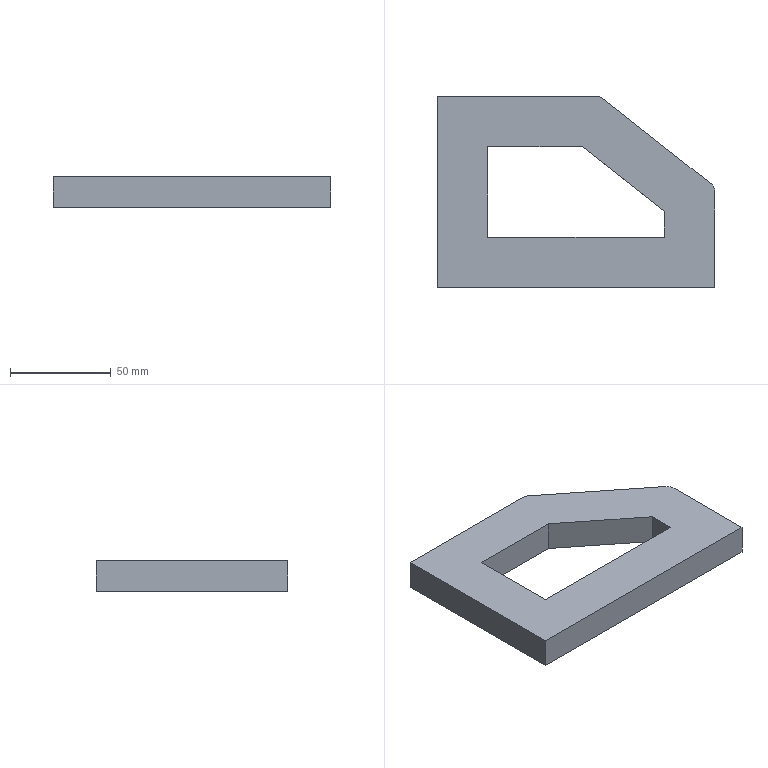Part | STEP file | ASND-0110-Part 14989898 | 1 solid | 16 faces | box 137.7 x 95 x 15 mm | volume 127568 mm3 | plane 12 | cylinder 4 | commonest cylinder face diameters 10 x4
STEP:
#1=CARTESIAN_POINT('',(0.,0.,0.));
#2=DIRECTION('',(0.,0.,1.));
#3=DIRECTION('',(1.,0.,0.));
#4=AXIS2_PLACEMENT_3D('',#1,#2,#3);
#5=CARTESIAN_POINT('',(78.964,95.,15.));
#6=VERTEX_POINT('',#5);
#7=CARTESIAN_POINT('',(80.604,94.723,15.));
#8=VERTEX_POINT('',#7);
#9=CARTESIAN_POINT('',(78.964,90.,15.));
#10=DIRECTION('',(0.,0.,-1.));
#11=DIRECTION('',(0.328,0.9447,0.));
#12=AXIS2_PLACEMENT_3D('',#9,#10,#11);
#13=CIRCLE('',#12,5.);
#14=CARTESIAN_POINT('',(78.964,90.,20.));
#15=DIRECTION('',(0.,0.,-1.));
#16=DIRECTION('',(0.328,0.9447,0.));
#17=AXIS2_PLACEMENT_3D('',#14,#15,#16);
#18=CYLINDRICAL_SURFACE('',#17,5.);
#19=CARTESIAN_POINT('',(0.,5.));
#20=DIRECTION('',(1.,0.));
#21=VECTOR('',#20,1.);
#22=LINE('',#19,#21);
#23=(GEOMETRIC_REPRESENTATION_CONTEXT(2)PARAMETRIC_REPRESENTATION_CONTEXT()REPRESENTATION_CONTEXT('',''));
#24=DEFINITIONAL_REPRESENTATION('',(#22),#23);
#25=PCURVE('',#18,#24);
#26=CARTESIAN_POINT('',(0.,0.,15.));
#27=DIRECTION('',(0.,0.,-1.));
#28=DIRECTION('',(0.7071,0.7071,0.));
#29=AXIS2_PLACEMENT_3D('',#26,#27,#28);
#30=PLANE('',#29);
#31=CARTESIAN_POINT('',(119.476,-7.803));
#32=DIRECTION('',(0.8999,-0.4361));
#33=AXIS2_PLACEMENT_2D('',#31,#32);
#34=CIRCLE('',#33,5.);
#35=(GEOMETRIC_REPRESENTATION_CONTEXT(2)PARAMETRIC_REPRESENTATION_CONTEXT()REPRESENTATION_CONTEXT('',''));
#36=DEFINITIONAL_REPRESENTATION('',(#34),#35);
#37=PCURVE('',#30,#36);
#38=SURFACE_CURVE('',#13,(#25,#37),.PCURVE_S1.);
#39=EDGE_CURVE('',#6,#8,#38,.T.);
#40=ORIENTED_EDGE('',*,*,#39,.T.);
#41=CARTESIAN_POINT('',(80.604,94.723,0.));
#42=VERTEX_POINT('',#41);
#43=CARTESIAN_POINT('',(80.604,94.723,20.));
#44=DIRECTION('',(0.,0.,-1.));
#45=VECTOR('',#44,1.);
#46=LINE('',#43,#45);
#47=CARTESIAN_POINT('',(6.283,0.));
#48=DIRECTION('',(0.,1.));
#49=VECTOR('',#48,1.);
#50=LINE('',#47,#49);
#51=(GEOMETRIC_REPRESENTATION_CONTEXT(2)PARAMETRIC_REPRESENTATION_CONTEXT()REPRESENTATION_CONTEXT('',''));
#52=DEFINITIONAL_REPRESENTATION('',(#50),#51);
#53=PCURVE('',#18,#52);
#54=CARTESIAN_POINT('',(78.964,90.,20.));
#55=DIRECTION('',(0.,0.,-1.));
#56=DIRECTION('',(0.328,0.9447,0.));
#57=AXIS2_PLACEMENT_3D('',#54,#55,#56);
#58=CYLINDRICAL_SURFACE('',#57,5.);
#59=CARTESIAN_POINT('',(0.,0.));
#60=DIRECTION('',(0.,1.));
#61=VECTOR('',#60,1.);
#62=LINE('',#59,#61);
#63=(GEOMETRIC_REPRESENTATION_CONTEXT(2)PARAMETRIC_REPRESENTATION_CONTEXT()REPRESENTATION_CONTEXT('',''));
#64=DEFINITIONAL_REPRESENTATION('',(#62),#63);
#65=PCURVE('',#58,#64);
#66=SURFACE_CURVE('',#46,(#53,#65),.PCURVE_S1.);
#67=EDGE_CURVE('',#8,#42,#66,.T.);
#68=ORIENTED_EDGE('',*,*,#67,.T.);
#69=CARTESIAN_POINT('',(78.964,95.,0.));
#70=VERTEX_POINT('',#69);
#71=CARTESIAN_POINT('',(78.964,90.,0.));
#72=DIRECTION('',(0.,0.,1.));
#73=DIRECTION('',(0.328,0.9447,0.));
#74=AXIS2_PLACEMENT_3D('',#71,#72,#73);
#75=CIRCLE('',#74,5.);
#76=CARTESIAN_POINT('',(6.283,20.));
#77=DIRECTION('',(-1.,0.));
#78=VECTOR('',#77,1.);
#79=LINE('',#76,#78);
#80=(GEOMETRIC_REPRESENTATION_CONTEXT(2)PARAMETRIC_REPRESENTATION_CONTEXT()REPRESENTATION_CONTEXT('',''));
#81=DEFINITIONAL_REPRESENTATION('',(#79),#80);
#82=PCURVE('',#18,#81);
#83=CARTESIAN_POINT('',(0.,0.,0.));
#84=DIRECTION('',(0.,0.,-1.));
#85=DIRECTION('',(0.7071,0.7071,0.));
#86=AXIS2_PLACEMENT_3D('',#83,#84,#85);
#87=PLANE('',#86);
#88=CARTESIAN_POINT('',(123.975,-9.984));
#89=CARTESIAN_POINT('',(120.199,-17.777));
#90=CARTESIAN_POINT('',(115.338,-10.61));
#91=CARTESIAN_POINT('',(110.477,-3.443));
#92=CARTESIAN_POINT('',(119.114,-2.817));
#93=CARTESIAN_POINT('',(127.752,-2.191));
#94=CARTESIAN_POINT('',(123.975,-9.984));
#95=(BOUNDED_CURVE()B_SPLINE_CURVE(2,(#88,#89,#90,#91,#92,#93,#94),.UNSPECIFIED.,.T.,.F.)B_SPLINE_CURVE_WITH_KNOTS((1,2,2,2,2,1),(-2.094,0.,2.094,4.189,6.283,8.378),.UNSPECIFIED.)CURVE()GEOMETRIC_REPRESENTATION_ITEM()RATIONAL_B_SPLINE_CURVE((1.,0.5,1.,0.5,1.,0.5,1.))REPRESENTATION_ITEM(''));
#96=(GEOMETRIC_REPRESENTATION_CONTEXT(2)PARAMETRIC_REPRESENTATION_CONTEXT()REPRESENTATION_CONTEXT('',''));
#97=DEFINITIONAL_REPRESENTATION('',(#95),#96);
#98=PCURVE('',#87,#97);
#99=SURFACE_CURVE('',#75,(#82,#98),.PCURVE_S1.);
#100=EDGE_CURVE('',#42,#70,#99,.T.);
#101=ORIENTED_EDGE('',*,*,#100,.T.);
#102=CARTESIAN_POINT('',(78.964,95.,20.));
#103=DIRECTION('',(0.,0.,1.));
#104=VECTOR('',#103,1.);
#105=LINE('',#102,#104);
#106=CARTESIAN_POINT('',(5.949,0.));
#107=DIRECTION('',(0.,-1.));
#108=VECTOR('',#107,1.);
#109=LINE('',#106,#108);
#110=(GEOMETRIC_REPRESENTATION_CONTEXT(2)PARAMETRIC_REPRESENTATION_CONTEXT()REPRESENTATION_CONTEXT('',''));
#111=DEFINITIONAL_REPRESENTATION('',(#109),#110);
#112=PCURVE('',#18,#111);
#113=CARTESIAN_POINT('',(0.,95.,20.));
#114=DIRECTION('',(0.,-1.,0.));
#115=DIRECTION('',(0.7071,0.,0.7071));
#116=AXIS2_PLACEMENT_3D('',#113,#114,#115);
#117=PLANE('',#116);
#118=CARTESIAN_POINT('',(55.836,-55.836));
#119=DIRECTION('',(0.7071,0.7071));
#120=VECTOR('',#119,1.);
#121=LINE('',#118,#120);
#122=(GEOMETRIC_REPRESENTATION_CONTEXT(2)PARAMETRIC_REPRESENTATION_CONTEXT()REPRESENTATION_CONTEXT('',''));
#123=DEFINITIONAL_REPRESENTATION('',(#121),#122);
#124=PCURVE('',#117,#123);
#125=SURFACE_CURVE('',#105,(#112,#124),.PCURVE_S1.);
#126=EDGE_CURVE('',#70,#6,#125,.T.);
#127=ORIENTED_EDGE('',*,*,#126,.T.);
#128=EDGE_LOOP('',(#40,#68,#101,#127));
#129=FACE_BOUND('',#128,.T.);
#130=ADVANCED_FACE('',(#129),#18,.T.);
#131=CARTESIAN_POINT('',(135.798,51.501,15.));
#132=VERTEX_POINT('',#131);
#133=CARTESIAN_POINT('',(137.2,49.757,15.));
#134=VERTEX_POINT('',#133);
#135=CARTESIAN_POINT('',(132.7,47.577,15.));
#136=DIRECTION('',(0.,0.,-1.));
#137=DIRECTION('',(0.8999,0.4361,0.));
#138=AXIS2_PLACEMENT_3D('',#135,#136,#137);
#139=CIRCLE('',#138,5.);
#140=CARTESIAN_POINT('',(132.7,47.577,20.));
#141=DIRECTION('',(0.,0.,-1.));
#142=DIRECTION('',(0.8999,0.4361,0.));
#143=AXIS2_PLACEMENT_3D('',#140,#141,#142);
#144=CYLINDRICAL_SURFACE('',#143,5.);
#145=CARTESIAN_POINT('',(0.,5.));
#146=DIRECTION('',(1.,0.));
#147=VECTOR('',#146,1.);
#148=LINE('',#145,#147);
#149=(GEOMETRIC_REPRESENTATION_CONTEXT(2)PARAMETRIC_REPRESENTATION_CONTEXT()REPRESENTATION_CONTEXT('',''));
#150=DEFINITIONAL_REPRESENTATION('',(#148),#149);
#151=PCURVE('',#144,#150);
#152=CARTESIAN_POINT('',(127.475,60.191));
#153=DIRECTION('',(0.9447,0.328));
#154=AXIS2_PLACEMENT_2D('',#152,#153);
#155=CIRCLE('',#154,5.);
#156=(GEOMETRIC_REPRESENTATION_CONTEXT(2)PARAMETRIC_REPRESENTATION_CONTEXT()REPRESENTATION_CONTEXT('',''));
#157=DEFINITIONAL_REPRESENTATION('',(#155),#156);
#158=PCURVE('',#30,#157);
#159=SURFACE_CURVE('',#139,(#151,#158),.PCURVE_S1.);
#160=EDGE_CURVE('',#132,#134,#159,.T.);
#161=ORIENTED_EDGE('',*,*,#160,.T.);
#162=CARTESIAN_POINT('',(137.2,49.757,0.));
#163=VERTEX_POINT('',#162);
#164=CARTESIAN_POINT('',(137.2,49.757,20.));
#165=DIRECTION('',(0.,0.,-1.));
#166=VECTOR('',#165,1.);
#167=LINE('',#164,#166);
#168=CARTESIAN_POINT('',(6.283,0.));
#169=DIRECTION('',(0.,1.));
#170=VECTOR('',#169,1.);
#171=LINE('',#168,#170);
#172=(GEOMETRIC_REPRESENTATION_CONTEXT(2)PARAMETRIC_REPRESENTATION_CONTEXT()REPRESENTATION_CONTEXT('',''));
#173=DEFINITIONAL_REPRESENTATION('',(#171),#172);
#174=PCURVE('',#144,#173);
#175=CARTESIAN_POINT('',(132.7,47.577,20.));
#176=DIRECTION('',(0.,0.,-1.));
#177=DIRECTION('',(0.8999,0.4361,0.));
#178=AXIS2_PLACEMENT_3D('',#175,#176,#177);
#179=CYLINDRICAL_SURFACE('',#178,5.);
#180=CARTESIAN_POINT('',(0.,0.));
#181=DIRECTION('',(0.,1.));
#182=VECTOR('',#181,1.);
#183=LINE('',#180,#182);
#184=(GEOMETRIC_REPRESENTATION_CONTEXT(2)PARAMETRIC_REPRESENTATION_CONTEXT()REPRESENTATION_CONTEXT('',''));
#185=DEFINITIONAL_REPRESENTATION('',(#183),#184);
#186=PCURVE('',#179,#185);
#187=SURFACE_CURVE('',#167,(#174,#186),.PCURVE_S1.);
#188=EDGE_CURVE('',#134,#163,#187,.T.);
#189=ORIENTED_EDGE('',*,*,#188,.T.);
#190=CARTESIAN_POINT('',(135.798,51.501,0.));
#191=VERTEX_POINT('',#190);
#192=CARTESIAN_POINT('',(132.7,47.577,0.));
#193=DIRECTION('',(0.,0.,1.));
#194=DIRECTION('',(0.8999,0.4361,0.));
#195=AXIS2_PLACEMENT_3D('',#192,#193,#194);
#196=CIRCLE('',#195,5.);
#197=CARTESIAN_POINT('',(6.283,20.));
#198=DIRECTION('',(-1.,0.));
#199=VECTOR('',#198,1.);
#200=LINE('',#197,#199);
#201=(GEOMETRIC_REPRESENTATION_CONTEXT(2)PARAMETRIC_REPRESENTATION_CONTEXT()REPRESENTATION_CONTEXT('',''));
#202=DEFINITIONAL_REPRESENTATION('',(#200),#201);
#203=PCURVE('',#144,#202);
#204=CARTESIAN_POINT('',(132.199,61.831));
#205=CARTESIAN_POINT('',(135.039,53.65));
#206=CARTESIAN_POINT('',(126.533,55.281));
#207=CARTESIAN_POINT('',(118.028,56.911));
#208=CARTESIAN_POINT('',(123.693,63.462));
#209=CARTESIAN_POINT('',(129.358,70.012));
#210=CARTESIAN_POINT('',(132.199,61.831));
#211=(BOUNDED_CURVE()B_SPLINE_CURVE(2,(#204,#205,#206,#207,#208,#209,#210),.UNSPECIFIED.,.T.,.F.)B_SPLINE_CURVE_WITH_KNOTS((1,2,2,2,2,1),(-2.094,0.,2.094,4.189,6.283,8.378),.UNSPECIFIED.)CURVE()GEOMETRIC_REPRESENTATION_ITEM()RATIONAL_B_SPLINE_CURVE((1.,0.5,1.,0.5,1.,0.5,1.))REPRESENTATION_ITEM(''));
#212=(GEOMETRIC_REPRESENTATION_CONTEXT(2)PARAMETRIC_REPRESENTATION_CONTEXT()REPRESENTATION_CONTEXT('',''));
#213=DEFINITIONAL_REPRESENTATION('',(#211),#212);
#214=PCURVE('',#87,#213);
#215=SURFACE_CURVE('',#196,(#203,#214),.PCURVE_S1.);
#216=EDGE_CURVE('',#163,#191,#215,.T.);
#217=ORIENTED_EDGE('',*,*,#216,.T.);
#218=CARTESIAN_POINT('',(135.798,51.501,20.));
#219=DIRECTION('',(0.,0.,1.));
#220=VECTOR('',#219,1.);
#221=LINE('',#218,#220);
#222=CARTESIAN_POINT('',(5.832,0.));
#223=DIRECTION('',(0.,-1.));
#224=VECTOR('',#223,1.);
#225=LINE('',#222,#224);
#226=(GEOMETRIC_REPRESENTATION_CONTEXT(2)PARAMETRIC_REPRESENTATION_CONTEXT()REPRESENTATION_CONTEXT('',''));
#227=DEFINITIONAL_REPRESENTATION('',(#225),#226);
#228=PCURVE('',#144,#227);
#229=CARTESIAN_POINT('',(-52.3,200.,20.));
#230=DIRECTION('',(-0.6196,-0.7849,0.));
#231=DIRECTION('',(-0.6672,0.5267,0.5267));
#232=AXIS2_PLACEMENT_3D('',#229,#230,#231);
#233=PLANE('',#232);
#234=CARTESIAN_POINT('',(-203.713,-126.229));
#235=DIRECTION('',(0.5267,-0.85));
#236=VECTOR('',#235,1.);
#237=LINE('',#234,#236);
#238=(GEOMETRIC_REPRESENTATION_CONTEXT(2)PARAMETRIC_REPRESENTATION_CONTEXT()REPRESENTATION_CONTEXT('',''));
#239=DEFINITIONAL_REPRESENTATION('',(#237),#238);
#240=PCURVE('',#233,#239);
#241=SURFACE_CURVE('',#221,(#228,#240),.PCURVE_S1.);
#242=EDGE_CURVE('',#191,#132,#241,.T.);
#243=ORIENTED_EDGE('',*,*,#242,.T.);
#244=EDGE_LOOP('',(#161,#189,#217,#243));
#245=FACE_BOUND('',#244,.T.);
#246=ADVANCED_FACE('',(#245),#144,.T.);
#247=ORIENTED_EDGE('',*,*,#188,.F.);
#248=CARTESIAN_POINT('',(137.7,47.577,15.));
#249=VERTEX_POINT('',#248);
#250=CARTESIAN_POINT('',(132.7,47.577,15.));
#251=DIRECTION('',(0.,0.,-1.));
#252=DIRECTION('',(0.8999,0.4361,0.));
#253=AXIS2_PLACEMENT_3D('',#250,#251,#252);
#254=CIRCLE('',#253,5.);
#255=CARTESIAN_POINT('',(0.,5.));
#256=DIRECTION('',(1.,0.));
#257=VECTOR('',#256,1.);
#258=LINE('',#255,#257);
#259=(GEOMETRIC_REPRESENTATION_CONTEXT(2)PARAMETRIC_REPRESENTATION_CONTEXT()REPRESENTATION_CONTEXT('',''));
#260=DEFINITIONAL_REPRESENTATION('',(#258),#259);
#261=PCURVE('',#179,#260);
#262=CARTESIAN_POINT('',(127.475,60.191));
#263=DIRECTION('',(0.9447,0.328));
#264=AXIS2_PLACEMENT_2D('',#262,#263);
#265=CIRCLE('',#264,5.);
#266=(GEOMETRIC_REPRESENTATION_CONTEXT(2)PARAMETRIC_REPRESENTATION_CONTEXT()REPRESENTATION_CONTEXT('',''));
#267=DEFINITIONAL_REPRESENTATION('',(#265),#266);
#268=PCURVE('',#30,#267);
#269=SURFACE_CURVE('',#254,(#261,#268),.PCURVE_S1.);
#270=EDGE_CURVE('',#134,#249,#269,.T.);
#271=ORIENTED_EDGE('',*,*,#270,.T.);
#272=CARTESIAN_POINT('',(137.7,47.577,0.));
#273=VERTEX_POINT('',#272);
#274=CARTESIAN_POINT('',(137.7,47.577,20.));
#275=DIRECTION('',(0.,0.,-1.));
#276=VECTOR('',#275,1.);
#277=LINE('',#274,#276);
#278=CARTESIAN_POINT('',(0.4513,0.));
#279=DIRECTION('',(0.,1.));
#280=VECTOR('',#279,1.);
#281=LINE('',#278,#280);
#282=(GEOMETRIC_REPRESENTATION_CONTEXT(2)PARAMETRIC_REPRESENTATION_CONTEXT()REPRESENTATION_CONTEXT('',''));
#283=DEFINITIONAL_REPRESENTATION('',(#281),#282);
#284=PCURVE('',#179,#283);
#285=CARTESIAN_POINT('',(137.7,50.,20.));
#286=DIRECTION('',(-1.,0.,0.));
#287=DIRECTION('',(0.,0.7071,0.7071));
#288=AXIS2_PLACEMENT_3D('',#285,#286,#287);
#289=PLANE('',#288);
#290=CARTESIAN_POINT('',(-1.713,-1.713));
#291=DIRECTION('',(-0.7071,0.7071));
#292=VECTOR('',#291,1.);
#293=LINE('',#290,#292);
#294=(GEOMETRIC_REPRESENTATION_CONTEXT(2)PARAMETRIC_REPRESENTATION_CONTEXT()REPRESENTATION_CONTEXT('',''));
#295=DEFINITIONAL_REPRESENTATION('',(#293),#294);
#296=PCURVE('',#289,#295);
#297=SURFACE_CURVE('',#277,(#284,#296),.PCURVE_S1.);
#298=EDGE_CURVE('',#249,#273,#297,.T.);
#299=ORIENTED_EDGE('',*,*,#298,.T.);
#300=CARTESIAN_POINT('',(132.7,47.577,0.));
#301=DIRECTION('',(0.,0.,1.));
#302=DIRECTION('',(0.8999,0.4361,0.));
#303=AXIS2_PLACEMENT_3D('',#300,#301,#302);
#304=CIRCLE('',#303,5.);
#305=CARTESIAN_POINT('',(6.283,20.));
#306=DIRECTION('',(-1.,0.));
#307=VECTOR('',#306,1.);
#308=LINE('',#305,#307);
#309=(GEOMETRIC_REPRESENTATION_CONTEXT(2)PARAMETRIC_REPRESENTATION_CONTEXT()REPRESENTATION_CONTEXT('',''));
#310=DEFINITIONAL_REPRESENTATION('',(#308),#309);
#311=PCURVE('',#179,#310);
#312=CARTESIAN_POINT('',(132.199,61.831));
#313=CARTESIAN_POINT('',(135.039,53.65));
#314=CARTESIAN_POINT('',(126.533,55.281));
#315=CARTESIAN_POINT('',(118.028,56.911));
#316=CARTESIAN_POINT('',(123.693,63.462));
#317=CARTESIAN_POINT('',(129.358,70.012));
#318=CARTESIAN_POINT('',(132.199,61.831));
#319=(BOUNDED_CURVE()B_SPLINE_CURVE(2,(#312,#313,#314,#315,#316,#317,#318),.UNSPECIFIED.,.T.,.F.)B_SPLINE_CURVE_WITH_KNOTS((1,2,2,2,2,1),(-2.094,0.,2.094,4.189,6.283,8.378),.UNSPECIFIED.)CURVE()GEOMETRIC_REPRESENTATION_ITEM()RATIONAL_B_SPLINE_CURVE((1.,0.5,1.,0.5,1.,0.5,1.))REPRESENTATION_ITEM(''));
#320=(GEOMETRIC_REPRESENTATION_CONTEXT(2)PARAMETRIC_REPRESENTATION_CONTEXT()REPRESENTATION_CONTEXT('',''));
#321=DEFINITIONAL_REPRESENTATION('',(#319),#320);
#322=PCURVE('',#87,#321);
#323=SURFACE_CURVE('',#304,(#311,#322),.PCURVE_S1.);
#324=EDGE_CURVE('',#273,#163,#323,.T.);
#325=ORIENTED_EDGE('',*,*,#324,.T.);
#326=EDGE_LOOP('',(#247,#271,#299,#325));
#327=FACE_BOUND('',#326,.T.);
#328=ADVANCED_FACE('',(#327),#179,.T.);
#329=ORIENTED_EDGE('',*,*,#298,.F.);
#330=CARTESIAN_POINT('',(137.7,0.,15.));
#331=VERTEX_POINT('',#330);
#332=CARTESIAN_POINT('',(137.7,0.,15.));
#333=DIRECTION('',(0.,1.,0.));
#334=VECTOR('',#333,1.);
#335=LINE('',#332,#334);
#336=CARTESIAN_POINT('',(-38.891,-31.82));
#337=DIRECTION('',(0.7071,0.7071));
#338=VECTOR('',#337,1.);
#339=LINE('',#336,#338);
#340=(GEOMETRIC_REPRESENTATION_CONTEXT(2)PARAMETRIC_REPRESENTATION_CONTEXT()REPRESENTATION_CONTEXT('',''));
#341=DEFINITIONAL_REPRESENTATION('',(#339),#340);
#342=PCURVE('',#289,#341);
#343=CARTESIAN_POINT('',(97.369,97.369));
#344=DIRECTION('',(0.7071,-0.7071));
#345=VECTOR('',#344,1.);
#346=LINE('',#343,#345);
#347=(GEOMETRIC_REPRESENTATION_CONTEXT(2)PARAMETRIC_REPRESENTATION_CONTEXT()REPRESENTATION_CONTEXT('',''));
#348=DEFINITIONAL_REPRESENTATION('',(#346),#347);
#349=PCURVE('',#30,#348);
#350=SURFACE_CURVE('',#335,(#342,#349),.PCURVE_S1.);
#351=EDGE_CURVE('',#331,#249,#350,.T.);
#352=ORIENTED_EDGE('',*,*,#351,.F.);
#353=CARTESIAN_POINT('',(137.7,0.,0.));
#354=VERTEX_POINT('',#353);
#355=CARTESIAN_POINT('',(137.7,0.,20.));
#356=DIRECTION('',(0.,0.,-1.));
#357=VECTOR('',#356,1.);
#358=LINE('',#355,#357);
#359=CARTESIAN_POINT('',(-35.355,-35.355));
#360=DIRECTION('',(-0.7071,0.7071));
#361=VECTOR('',#360,1.);
#362=LINE('',#359,#361);
#363=(GEOMETRIC_REPRESENTATION_CONTEXT(2)PARAMETRIC_REPRESENTATION_CONTEXT()REPRESENTATION_CONTEXT('',''));
#364=DEFINITIONAL_REPRESENTATION('',(#362),#363);
#365=PCURVE('',#289,#364);
#366=CARTESIAN_POINT('',(220.,0.,20.));
#367=DIRECTION('',(0.,1.,0.));
#368=DIRECTION('',(0.7071,0.,0.7071));
#369=AXIS2_PLACEMENT_3D('',#366,#367,#368);
#370=PLANE('',#369);
#371=CARTESIAN_POINT('',(-58.195,-58.195));
#372=DIRECTION('',(-0.7071,0.7071));
#373=VECTOR('',#372,1.);
#374=LINE('',#371,#373);
#375=(GEOMETRIC_REPRESENTATION_CONTEXT(2)PARAMETRIC_REPRESENTATION_CONTEXT()REPRESENTATION_CONTEXT('',''));
#376=DEFINITIONAL_REPRESENTATION('',(#374),#375);
#377=PCURVE('',#370,#376);
#378=SURFACE_CURVE('',#358,(#365,#377),.PCURVE_S1.);
#379=EDGE_CURVE('',#331,#354,#378,.T.);
#380=ORIENTED_EDGE('',*,*,#379,.T.);
#381=CARTESIAN_POINT('',(137.7,0.,0.));
#382=DIRECTION('',(0.,1.,0.));
#383=VECTOR('',#382,1.);
#384=LINE('',#381,#383);
#385=CARTESIAN_POINT('',(-49.497,-21.213));
#386=DIRECTION('',(0.7071,0.7071));
#387=VECTOR('',#386,1.);
#388=LINE('',#385,#387);
#389=(GEOMETRIC_REPRESENTATION_CONTEXT(2)PARAMETRIC_REPRESENTATION_CONTEXT()REPRESENTATION_CONTEXT('',''));
#390=DEFINITIONAL_REPRESENTATION('',(#388),#389);
#391=PCURVE('',#289,#390);
#392=CARTESIAN_POINT('',(97.369,97.369));
#393=DIRECTION('',(0.7071,-0.7071));
#394=VECTOR('',#393,1.);
#395=LINE('',#392,#394);
#396=(GEOMETRIC_REPRESENTATION_CONTEXT(2)PARAMETRIC_REPRESENTATION_CONTEXT()REPRESENTATION_CONTEXT('',''));
#397=DEFINITIONAL_REPRESENTATION('',(#395),#396);
#398=PCURVE('',#87,#397);
#399=SURFACE_CURVE('',#384,(#391,#398),.PCURVE_S1.);
#400=EDGE_CURVE('',#354,#273,#399,.T.);
#401=ORIENTED_EDGE('',*,*,#400,.T.);
#402=EDGE_LOOP('',(#329,#352,#380,#401));
#403=FACE_BOUND('',#402,.T.);
#404=ADVANCED_FACE('',(#403),#289,.F.);
#405=CARTESIAN_POINT('',(72.021,70.,15.));
#406=VERTEX_POINT('',#405);
#407=CARTESIAN_POINT('',(112.7,37.885,15.));
#408=VERTEX_POINT('',#407);
#409=CARTESIAN_POINT('',(40.354,95.,15.));
#410=DIRECTION('',(0.7849,-0.6196,0.));
#411=VECTOR('',#410,1.);
#412=LINE('',#409,#411);
#413=CARTESIAN_POINT('',(95.71,-38.64));
#414=DIRECTION('',(0.1168,0.9932));
#415=VECTOR('',#414,1.);
#416=LINE('',#413,#415);
#417=(GEOMETRIC_REPRESENTATION_CONTEXT(2)PARAMETRIC_REPRESENTATION_CONTEXT()REPRESENTATION_CONTEXT('',''));
#418=DEFINITIONAL_REPRESENTATION('',(#416),#417);
#419=PCURVE('',#30,#418);
#420=CARTESIAN_POINT('',(2.354,125.,0.));
#421=DIRECTION('',(0.6196,0.7849,0.));
#422=DIRECTION('',(-0.6672,0.5267,0.5267));
#423=AXIS2_PLACEMENT_3D('',#420,#421,#422);
#424=PLANE('',#423);
#425=CARTESIAN_POINT('',(-33.254,38.252));
#426=DIRECTION('',(-0.85,0.5267));
#427=VECTOR('',#426,1.);
#428=LINE('',#425,#427);
#429=(GEOMETRIC_REPRESENTATION_CONTEXT(2)PARAMETRIC_REPRESENTATION_CONTEXT()REPRESENTATION_CONTEXT('',''));
#430=DEFINITIONAL_REPRESENTATION('',(#428),#429);
#431=PCURVE('',#424,#430);
#432=SURFACE_CURVE('',#412,(#419,#431),.PCURVE_S1.);
#433=EDGE_CURVE('',#406,#408,#432,.T.);
#434=ORIENTED_EDGE('',*,*,#433,.T.);
#435=CARTESIAN_POINT('',(112.7,25.,15.));
#436=VERTEX_POINT('',#435);
#437=CARTESIAN_POINT('',(112.7,37.885,15.));
#438=DIRECTION('',(0.,-1.,0.));
#439=VECTOR('',#438,1.);
#440=LINE('',#437,#439);
#441=CARTESIAN_POINT('',(106.48,52.902));
#442=DIRECTION('',(-0.7071,0.7071));
#443=VECTOR('',#442,1.);
#444=LINE('',#441,#443);
#445=(GEOMETRIC_REPRESENTATION_CONTEXT(2)PARAMETRIC_REPRESENTATION_CONTEXT()REPRESENTATION_CONTEXT('',''));
#446=DEFINITIONAL_REPRESENTATION('',(#444),#445);
#447=PCURVE('',#30,#446);
#448=CARTESIAN_POINT('',(112.7,37.885,0.));
#449=DIRECTION('',(1.,0.,0.));
#450=DIRECTION('',(0.,0.7071,0.7071));
#451=AXIS2_PLACEMENT_3D('',#448,#449,#450);
#452=PLANE('',#451);
#453=CARTESIAN_POINT('',(10.607,10.607));
#454=DIRECTION('',(-0.7071,0.7071));
#455=VECTOR('',#454,1.);
#456=LINE('',#453,#455);
#457=(GEOMETRIC_REPRESENTATION_CONTEXT(2)PARAMETRIC_REPRESENTATION_CONTEXT()REPRESENTATION_CONTEXT('',''));
#458=DEFINITIONAL_REPRESENTATION('',(#456),#457);
#459=PCURVE('',#452,#458);
#460=SURFACE_CURVE('',#440,(#447,#459),.PCURVE_S1.);
#461=EDGE_CURVE('',#408,#436,#460,.T.);
#462=ORIENTED_EDGE('',*,*,#461,.T.);
#463=CARTESIAN_POINT('',(25.,25.,15.));
#464=VERTEX_POINT('',#463);
#465=CARTESIAN_POINT('',(195.,25.,15.));
#466=DIRECTION('',(-1.,0.,0.));
#467=VECTOR('',#466,1.);
#468=LINE('',#465,#467);
#469=CARTESIAN_POINT('',(155.563,120.208));
#470=DIRECTION('',(-0.7071,-0.7071));
#471=VECTOR('',#470,1.);
#472=LINE('',#469,#471);
#473=(GEOMETRIC_REPRESENTATION_CONTEXT(2)PARAMETRIC_REPRESENTATION_CONTEXT()REPRESENTATION_CONTEXT('',''));
#474=DEFINITIONAL_REPRESENTATION('',(#472),#473);
#475=PCURVE('',#30,#474);
#476=CARTESIAN_POINT('',(195.,25.,0.));
#477=DIRECTION('',(0.,-1.,0.));
#478=DIRECTION('',(0.7071,0.,0.7071));
#479=AXIS2_PLACEMENT_3D('',#476,#477,#478);
#480=PLANE('',#479);
#481=CARTESIAN_POINT('',(10.607,10.607));
#482=DIRECTION('',(-0.7071,0.7071));
#483=VECTOR('',#482,1.);
#484=LINE('',#481,#483);
#485=(GEOMETRIC_REPRESENTATION_CONTEXT(2)PARAMETRIC_REPRESENTATION_CONTEXT()REPRESENTATION_CONTEXT('',''));
#486=DEFINITIONAL_REPRESENTATION('',(#484),#485);
#487=PCURVE('',#480,#486);
#488=SURFACE_CURVE('',#468,(#475,#487),.PCURVE_S1.);
#489=EDGE_CURVE('',#436,#464,#488,.T.);
#490=ORIENTED_EDGE('',*,*,#489,.T.);
#491=CARTESIAN_POINT('',(25.,70.,15.));
#492=VERTEX_POINT('',#491);
#493=CARTESIAN_POINT('',(25.,25.,15.));
#494=DIRECTION('',(0.,1.,0.));
#495=VECTOR('',#494,1.);
#496=LINE('',#493,#495);
#497=CARTESIAN_POINT('',(35.355,0.));
#498=DIRECTION('',(0.7071,-0.7071));
#499=VECTOR('',#498,1.);
#500=LINE('',#497,#499);
#501=(GEOMETRIC_REPRESENTATION_CONTEXT(2)PARAMETRIC_REPRESENTATION_CONTEXT()REPRESENTATION_CONTEXT('',''));
#502=DEFINITIONAL_REPRESENTATION('',(#500),#501);
#503=PCURVE('',#30,#502);
#504=CARTESIAN_POINT('',(25.,25.,0.));
#505=DIRECTION('',(-1.,0.,0.));
#506=DIRECTION('',(0.,0.7071,0.7071));
#507=AXIS2_PLACEMENT_3D('',#504,#505,#506);
#508=PLANE('',#507);
#509=CARTESIAN_POINT('',(10.607,-10.607));
#510=DIRECTION('',(0.7071,0.7071));
#511=VECTOR('',#510,1.);
#512=LINE('',#509,#511);
#513=(GEOMETRIC_REPRESENTATION_CONTEXT(2)PARAMETRIC_REPRESENTATION_CONTEXT()REPRESENTATION_CONTEXT('',''));
#514=DEFINITIONAL_REPRESENTATION('',(#512),#513);
#515=PCURVE('',#508,#514);
#516=SURFACE_CURVE('',#496,(#503,#515),.PCURVE_S1.);
#517=EDGE_CURVE('',#464,#492,#516,.T.);
#518=ORIENTED_EDGE('',*,*,#517,.T.);
#519=CARTESIAN_POINT('',(25.,70.,15.));
#520=DIRECTION('',(1.,0.,0.));
#521=VECTOR('',#520,1.);
#522=LINE('',#519,#521);
#523=CARTESIAN_POINT('',(67.175,-31.82));
#524=DIRECTION('',(0.7071,0.7071));
#525=VECTOR('',#524,1.);
#526=LINE('',#523,#525);
#527=(GEOMETRIC_REPRESENTATION_CONTEXT(2)PARAMETRIC_REPRESENTATION_CONTEXT()REPRESENTATION_CONTEXT('',''));
#528=DEFINITIONAL_REPRESENTATION('',(#526),#527);
#529=PCURVE('',#30,#528);
#530=CARTESIAN_POINT('',(25.,70.,0.));
#531=DIRECTION('',(0.,1.,0.));
#532=DIRECTION('',(0.7071,0.,0.7071));
#533=AXIS2_PLACEMENT_3D('',#530,#531,#532);
#534=PLANE('',#533);
#535=CARTESIAN_POINT('',(10.607,-10.607));
#536=DIRECTION('',(0.7071,0.7071));
#537=VECTOR('',#536,1.);
#538=LINE('',#535,#537);
#539=(GEOMETRIC_REPRESENTATION_CONTEXT(2)PARAMETRIC_REPRESENTATION_CONTEXT()REPRESENTATION_CONTEXT('',''));
#540=DEFINITIONAL_REPRESENTATION('',(#538),#539);
#541=PCURVE('',#534,#540);
#542=SURFACE_CURVE('',#522,(#529,#541),.PCURVE_S1.);
#543=EDGE_CURVE('',#492,#406,#542,.T.);
#544=ORIENTED_EDGE('',*,*,#543,.T.);
#545=EDGE_LOOP('',(#434,#462,#490,#518,#544));
#546=FACE_BOUND('',#545,.T.);
#547=ORIENTED_EDGE('',*,*,#160,.F.);
#548=CARTESIAN_POINT('',(82.062,93.924,15.));
#549=VERTEX_POINT('',#548);
#550=CARTESIAN_POINT('',(137.7,50.,15.));
#551=DIRECTION('',(-0.7849,0.6196,0.));
#552=VECTOR('',#551,1.);
#553=LINE('',#550,#552);
#554=CARTESIAN_POINT('',(132.724,62.013));
#555=DIRECTION('',(-0.1168,-0.9932));
#556=VECTOR('',#555,1.);
#557=LINE('',#554,#556);
#558=(GEOMETRIC_REPRESENTATION_CONTEXT(2)PARAMETRIC_REPRESENTATION_CONTEXT()REPRESENTATION_CONTEXT('',''));
#559=DEFINITIONAL_REPRESENTATION('',(#557),#558);
#560=PCURVE('',#30,#559);
#561=CARTESIAN_POINT('',(-208.406,-123.256));
#562=DIRECTION('',(0.85,0.5267));
#563=VECTOR('',#562,1.);
#564=LINE('',#561,#563);
#565=(GEOMETRIC_REPRESENTATION_CONTEXT(2)PARAMETRIC_REPRESENTATION_CONTEXT()REPRESENTATION_CONTEXT('',''));
#566=DEFINITIONAL_REPRESENTATION('',(#564),#565);
#567=PCURVE('',#233,#566);
#568=SURFACE_CURVE('',#553,(#560,#567),.PCURVE_S1.);
#569=EDGE_CURVE('',#132,#549,#568,.T.);
#570=ORIENTED_EDGE('',*,*,#569,.T.);
#571=CARTESIAN_POINT('',(78.964,90.,15.));
#572=DIRECTION('',(0.,0.,-1.));
#573=DIRECTION('',(0.328,0.9447,0.));
#574=AXIS2_PLACEMENT_3D('',#571,#572,#573);
#575=CIRCLE('',#574,5.);
#576=CARTESIAN_POINT('',(119.476,-7.803));
#577=DIRECTION('',(0.8999,-0.4361));
#578=AXIS2_PLACEMENT_2D('',#576,#577);
#579=CIRCLE('',#578,5.);
#580=(GEOMETRIC_REPRESENTATION_CONTEXT(2)PARAMETRIC_REPRESENTATION_CONTEXT()REPRESENTATION_CONTEXT('',''));
#581=DEFINITIONAL_REPRESENTATION('',(#579),#580);
#582=PCURVE('',#30,#581);
#583=CARTESIAN_POINT('',(0.,5.));
#584=DIRECTION('',(1.,0.));
#585=VECTOR('',#584,1.);
#586=LINE('',#583,#585);
#587=(GEOMETRIC_REPRESENTATION_CONTEXT(2)PARAMETRIC_REPRESENTATION_CONTEXT()REPRESENTATION_CONTEXT('',''));
#588=DEFINITIONAL_REPRESENTATION('',(#586),#587);
#589=PCURVE('',#58,#588);
#590=SURFACE_CURVE('',#575,(#582,#589),.PCURVE_S1.);
#591=EDGE_CURVE('',#8,#549,#590,.T.);
#592=ORIENTED_EDGE('',*,*,#591,.F.);
#593=ORIENTED_EDGE('',*,*,#39,.F.);
#594=CARTESIAN_POINT('',(0.,95.,15.));
#595=VERTEX_POINT('',#594);
#596=CARTESIAN_POINT('',(131.333,95.,15.));
#597=DIRECTION('',(-1.,0.,0.));
#598=VECTOR('',#597,1.);
#599=LINE('',#596,#598);
#600=CARTESIAN_POINT('',(160.042,25.692));
#601=DIRECTION('',(-0.7071,-0.7071));
#602=VECTOR('',#601,1.);
#603=LINE('',#600,#602);
#604=(GEOMETRIC_REPRESENTATION_CONTEXT(2)PARAMETRIC_REPRESENTATION_CONTEXT()REPRESENTATION_CONTEXT('',''));
#605=DEFINITIONAL_REPRESENTATION('',(#603),#604);
#606=PCURVE('',#30,#605);
#607=CARTESIAN_POINT('',(89.331,-96.402));
#608=DIRECTION('',(-0.7071,0.7071));
#609=VECTOR('',#608,1.);
#610=LINE('',#607,#609);
#611=(GEOMETRIC_REPRESENTATION_CONTEXT(2)PARAMETRIC_REPRESENTATION_CONTEXT()REPRESENTATION_CONTEXT('',''));
#612=DEFINITIONAL_REPRESENTATION('',(#610),#611);
#613=PCURVE('',#117,#612);
#614=SURFACE_CURVE('',#599,(#606,#613),.PCURVE_S1.);
#615=EDGE_CURVE('',#6,#595,#614,.T.);
#616=ORIENTED_EDGE('',*,*,#615,.T.);
#617=CARTESIAN_POINT('',(0.,0.,15.));
#618=VERTEX_POINT('',#617);
#619=CARTESIAN_POINT('',(0.,120.,15.));
#620=DIRECTION('',(0.,-1.,0.));
#621=VECTOR('',#620,1.);
#622=LINE('',#619,#621);
#623=CARTESIAN_POINT('',(84.853,-84.853));
#624=DIRECTION('',(-0.7071,0.7071));
#625=VECTOR('',#624,1.);
#626=LINE('',#623,#625);
#627=(GEOMETRIC_REPRESENTATION_CONTEXT(2)PARAMETRIC_REPRESENTATION_CONTEXT()REPRESENTATION_CONTEXT('',''));
#628=DEFINITIONAL_REPRESENTATION('',(#626),#627);
#629=PCURVE('',#30,#628);
#630=CARTESIAN_POINT('',(0.,0.,20.));
#631=DIRECTION('',(1.,0.,0.));
#632=DIRECTION('',(0.,0.7071,0.7071));
#633=AXIS2_PLACEMENT_3D('',#630,#631,#632);
#634=PLANE('',#633);
#635=CARTESIAN_POINT('',(81.317,-88.388));
#636=DIRECTION('',(-0.7071,0.7071));
#637=VECTOR('',#636,1.);
#638=LINE('',#635,#637);
#639=(GEOMETRIC_REPRESENTATION_CONTEXT(2)PARAMETRIC_REPRESENTATION_CONTEXT()REPRESENTATION_CONTEXT('',''));
#640=DEFINITIONAL_REPRESENTATION('',(#638),#639);
#641=PCURVE('',#634,#640);
#642=SURFACE_CURVE('',#622,(#629,#641),.PCURVE_S1.);
#643=EDGE_CURVE('',#595,#618,#642,.T.);
#644=ORIENTED_EDGE('',*,*,#643,.T.);
#645=CARTESIAN_POINT('',(0.,0.,15.));
#646=DIRECTION('',(1.,0.,0.));
#647=VECTOR('',#646,1.);
#648=LINE('',#645,#647);
#649=CARTESIAN_POINT('',(0.,0.));
#650=DIRECTION('',(0.7071,0.7071));
#651=VECTOR('',#650,1.);
#652=LINE('',#649,#651);
#653=(GEOMETRIC_REPRESENTATION_CONTEXT(2)PARAMETRIC_REPRESENTATION_CONTEXT()REPRESENTATION_CONTEXT('',''));
#654=DEFINITIONAL_REPRESENTATION('',(#652),#653);
#655=PCURVE('',#30,#654);
#656=CARTESIAN_POINT('',(-159.099,-152.028));
#657=DIRECTION('',(0.7071,0.7071));
#658=VECTOR('',#657,1.);
#659=LINE('',#656,#658);
#660=(GEOMETRIC_REPRESENTATION_CONTEXT(2)PARAMETRIC_REPRESENTATION_CONTEXT()REPRESENTATION_CONTEXT('',''));
#661=DEFINITIONAL_REPRESENTATION('',(#659),#660);
#662=PCURVE('',#370,#661);
#663=SURFACE_CURVE('',#648,(#655,#662),.PCURVE_S1.);
#664=EDGE_CURVE('',#618,#331,#663,.T.);
#665=ORIENTED_EDGE('',*,*,#664,.T.);
#666=ORIENTED_EDGE('',*,*,#351,.T.);
#667=ORIENTED_EDGE('',*,*,#270,.F.);
#668=EDGE_LOOP('',(#547,#570,#592,#593,#616,#644,#665,#666,#667));
#669=FACE_BOUND('',#668,.T.);
#670=ADVANCED_FACE('',(#546,#669),#30,.F.);
#671=ORIENTED_EDGE('',*,*,#67,.F.);
#672=ORIENTED_EDGE('',*,*,#591,.T.);
#673=CARTESIAN_POINT('',(82.062,93.924,0.));
#674=VERTEX_POINT('',#673);
#675=CARTESIAN_POINT('',(82.062,93.924,20.));
#676=DIRECTION('',(0.,0.,-1.));
#677=VECTOR('',#676,1.);
#678=LINE('',#675,#677);
#679=CARTESIAN_POINT('',(0.3341,0.));
#680=DIRECTION('',(0.,1.));
#681=VECTOR('',#680,1.);
#682=LINE('',#679,#681);
#683=(GEOMETRIC_REPRESENTATION_CONTEXT(2)PARAMETRIC_REPRESENTATION_CONTEXT()REPRESENTATION_CONTEXT('',''));
#684=DEFINITIONAL_REPRESENTATION('',(#682),#683);
#685=PCURVE('',#58,#684);
#686=CARTESIAN_POINT('',(-145.516,-90.168));
#687=DIRECTION('',(-0.5267,0.85));
#688=VECTOR('',#687,1.);
#689=LINE('',#686,#688);
#690=(GEOMETRIC_REPRESENTATION_CONTEXT(2)PARAMETRIC_REPRESENTATION_CONTEXT()REPRESENTATION_CONTEXT('',''));
#691=DEFINITIONAL_REPRESENTATION('',(#689),#690);
#692=PCURVE('',#233,#691);
#693=SURFACE_CURVE('',#678,(#685,#692),.PCURVE_S1.);
#694=EDGE_CURVE('',#549,#674,#693,.T.);
#695=ORIENTED_EDGE('',*,*,#694,.T.);
#696=CARTESIAN_POINT('',(78.964,90.,0.));
#697=DIRECTION('',(0.,0.,1.));
#698=DIRECTION('',(0.328,0.9447,0.));
#699=AXIS2_PLACEMENT_3D('',#696,#697,#698);
#700=CIRCLE('',#699,5.);
#701=CARTESIAN_POINT('',(6.283,20.));
#702=DIRECTION('',(-1.,0.));
#703=VECTOR('',#702,1.);
#704=LINE('',#701,#703);
#705=(GEOMETRIC_REPRESENTATION_CONTEXT(2)PARAMETRIC_REPRESENTATION_CONTEXT()REPRESENTATION_CONTEXT('',''));
#706=DEFINITIONAL_REPRESENTATION('',(#704),#705);
#707=PCURVE('',#58,#706);
#708=CARTESIAN_POINT('',(123.975,-9.984));
#709=CARTESIAN_POINT('',(120.199,-17.777));
#710=CARTESIAN_POINT('',(115.338,-10.61));
#711=CARTESIAN_POINT('',(110.477,-3.443));
#712=CARTESIAN_POINT('',(119.114,-2.817));
#713=CARTESIAN_POINT('',(127.752,-2.191));
#714=CARTESIAN_POINT('',(123.975,-9.984));
#715=(BOUNDED_CURVE()B_SPLINE_CURVE(2,(#708,#709,#710,#711,#712,#713,#714),.UNSPECIFIED.,.T.,.F.)B_SPLINE_CURVE_WITH_KNOTS((1,2,2,2,2,1),(-2.094,0.,2.094,4.189,6.283,8.378),.UNSPECIFIED.)CURVE()GEOMETRIC_REPRESENTATION_ITEM()RATIONAL_B_SPLINE_CURVE((1.,0.5,1.,0.5,1.,0.5,1.))REPRESENTATION_ITEM(''));
#716=(GEOMETRIC_REPRESENTATION_CONTEXT(2)PARAMETRIC_REPRESENTATION_CONTEXT()REPRESENTATION_CONTEXT('',''));
#717=DEFINITIONAL_REPRESENTATION('',(#715),#716);
#718=PCURVE('',#87,#717);
#719=SURFACE_CURVE('',#700,(#707,#718),.PCURVE_S1.);
#720=EDGE_CURVE('',#674,#42,#719,.T.);
#721=ORIENTED_EDGE('',*,*,#720,.T.);
#722=EDGE_LOOP('',(#671,#672,#695,#721));
#723=FACE_BOUND('',#722,.T.);
#724=ADVANCED_FACE('',(#723),#58,.T.);
#725=ORIENTED_EDGE('',*,*,#126,.F.);
#726=CARTESIAN_POINT('',(0.,95.,0.));
#727=VERTEX_POINT('',#726);
#728=CARTESIAN_POINT('',(131.333,95.,0.));
#729=DIRECTION('',(-1.,0.,0.));
#730=VECTOR('',#729,1.);
#731=LINE('',#728,#730);
#732=CARTESIAN_POINT('',(78.725,-107.009));
#733=DIRECTION('',(-0.7071,0.7071));
#734=VECTOR('',#733,1.);
#735=LINE('',#732,#734);
#736=(GEOMETRIC_REPRESENTATION_CONTEXT(2)PARAMETRIC_REPRESENTATION_CONTEXT()REPRESENTATION_CONTEXT('',''));
#737=DEFINITIONAL_REPRESENTATION('',(#735),#736);
#738=PCURVE('',#117,#737);
#739=CARTESIAN_POINT('',(160.042,25.692));
#740=DIRECTION('',(-0.7071,-0.7071));
#741=VECTOR('',#740,1.);
#742=LINE('',#739,#741);
#743=(GEOMETRIC_REPRESENTATION_CONTEXT(2)PARAMETRIC_REPRESENTATION_CONTEXT()REPRESENTATION_CONTEXT('',''));
#744=DEFINITIONAL_REPRESENTATION('',(#742),#743);
#745=PCURVE('',#87,#744);
#746=SURFACE_CURVE('',#731,(#738,#745),.PCURVE_S1.);
#747=EDGE_CURVE('',#70,#727,#746,.T.);
#748=ORIENTED_EDGE('',*,*,#747,.T.);
#749=CARTESIAN_POINT('',(0.,95.,20.));
#750=DIRECTION('',(0.,0.,-1.));
#751=VECTOR('',#750,1.);
#752=LINE('',#749,#751);
#753=CARTESIAN_POINT('',(0.,0.));
#754=DIRECTION('',(-0.7071,-0.7071));
#755=VECTOR('',#754,1.);
#756=LINE('',#753,#755);
#757=(GEOMETRIC_REPRESENTATION_CONTEXT(2)PARAMETRIC_REPRESENTATION_CONTEXT()REPRESENTATION_CONTEXT('',''));
#758=DEFINITIONAL_REPRESENTATION('',(#756),#757);
#759=PCURVE('',#117,#758);
#760=CARTESIAN_POINT('',(67.175,-67.175));
#761=DIRECTION('',(-0.7071,-0.7071));
#762=VECTOR('',#761,1.);
#763=LINE('',#760,#762);
#764=(GEOMETRIC_REPRESENTATION_CONTEXT(2)PARAMETRIC_REPRESENTATION_CONTEXT()REPRESENTATION_CONTEXT('',''));
#765=DEFINITIONAL_REPRESENTATION('',(#763),#764);
#766=PCURVE('',#634,#765);
#767=SURFACE_CURVE('',#752,(#759,#766),.PCURVE_S1.);
#768=EDGE_CURVE('',#595,#727,#767,.T.);
#769=ORIENTED_EDGE('',*,*,#768,.F.);
#770=ORIENTED_EDGE('',*,*,#615,.F.);
#771=EDGE_LOOP('',(#725,#748,#769,#770));
#772=FACE_BOUND('',#771,.T.);
#773=ADVANCED_FACE('',(#772),#117,.F.);
#774=ORIENTED_EDGE('',*,*,#324,.F.);
#775=ORIENTED_EDGE('',*,*,#400,.F.);
#776=CARTESIAN_POINT('',(0.,0.,0.));
#777=VERTEX_POINT('',#776);
#778=CARTESIAN_POINT('',(0.,0.,0.));
#779=DIRECTION('',(1.,0.,0.));
#780=VECTOR('',#779,1.);
#781=LINE('',#778,#780);
#782=CARTESIAN_POINT('',(0.,0.));
#783=DIRECTION('',(0.7071,0.7071));
#784=VECTOR('',#783,1.);
#785=LINE('',#782,#784);
#786=(GEOMETRIC_REPRESENTATION_CONTEXT(2)PARAMETRIC_REPRESENTATION_CONTEXT()REPRESENTATION_CONTEXT('',''));
#787=DEFINITIONAL_REPRESENTATION('',(#785),#786);
#788=PCURVE('',#87,#787);
#789=CARTESIAN_POINT('',(-169.706,-141.421));
#790=DIRECTION('',(0.7071,0.7071));
#791=VECTOR('',#790,1.);
#792=LINE('',#789,#791);
#793=(GEOMETRIC_REPRESENTATION_CONTEXT(2)PARAMETRIC_REPRESENTATION_CONTEXT()REPRESENTATION_CONTEXT('',''));
#794=DEFINITIONAL_REPRESENTATION('',(#792),#793);
#795=PCURVE('',#370,#794);
#796=SURFACE_CURVE('',#781,(#788,#795),.PCURVE_S1.);
#797=EDGE_CURVE('',#777,#354,#796,.T.);
#798=ORIENTED_EDGE('',*,*,#797,.F.);
#799=CARTESIAN_POINT('',(0.,120.,0.));
#800=DIRECTION('',(0.,-1.,0.));
#801=VECTOR('',#800,1.);
#802=LINE('',#799,#801);
#803=CARTESIAN_POINT('',(84.853,-84.853));
#804=DIRECTION('',(-0.7071,0.7071));
#805=VECTOR('',#804,1.);
#806=LINE('',#803,#805);
#807=(GEOMETRIC_REPRESENTATION_CONTEXT(2)PARAMETRIC_REPRESENTATION_CONTEXT()REPRESENTATION_CONTEXT('',''));
#808=DEFINITIONAL_REPRESENTATION('',(#806),#807);
#809=PCURVE('',#87,#808);
#810=CARTESIAN_POINT('',(70.711,-98.995));
#811=DIRECTION('',(-0.7071,0.7071));
#812=VECTOR('',#811,1.);
#813=LINE('',#810,#812);
#814=(GEOMETRIC_REPRESENTATION_CONTEXT(2)PARAMETRIC_REPRESENTATION_CONTEXT()REPRESENTATION_CONTEXT('',''));
#815=DEFINITIONAL_REPRESENTATION('',(#813),#814);
#816=PCURVE('',#634,#815);
#817=SURFACE_CURVE('',#802,(#809,#816),.PCURVE_S1.);
#818=EDGE_CURVE('',#727,#777,#817,.T.);
#819=ORIENTED_EDGE('',*,*,#818,.F.);
#820=ORIENTED_EDGE('',*,*,#747,.F.);
#821=ORIENTED_EDGE('',*,*,#100,.F.);
#822=ORIENTED_EDGE('',*,*,#720,.F.);
#823=CARTESIAN_POINT('',(137.7,50.,0.));
#824=DIRECTION('',(-0.7849,0.6196,0.));
#825=VECTOR('',#824,1.);
#826=LINE('',#823,#825);
#827=CARTESIAN_POINT('',(132.724,62.013));
#828=DIRECTION('',(-0.1168,-0.9932));
#829=VECTOR('',#828,1.);
#830=LINE('',#827,#829);
#831=(GEOMETRIC_REPRESENTATION_CONTEXT(2)PARAMETRIC_REPRESENTATION_CONTEXT()REPRESENTATION_CONTEXT('',''));
#832=DEFINITIONAL_REPRESENTATION('',(#830),#831);
#833=PCURVE('',#87,#832);
#834=CARTESIAN_POINT('',(-216.307,-110.505));
#835=DIRECTION('',(0.85,0.5267));
#836=VECTOR('',#835,1.);
#837=LINE('',#834,#836);
#838=(GEOMETRIC_REPRESENTATION_CONTEXT(2)PARAMETRIC_REPRESENTATION_CONTEXT()REPRESENTATION_CONTEXT('',''));
#839=DEFINITIONAL_REPRESENTATION('',(#837),#838);
#840=PCURVE('',#233,#839);
#841=SURFACE_CURVE('',#826,(#833,#840),.PCURVE_S1.);
#842=EDGE_CURVE('',#191,#674,#841,.T.);
#843=ORIENTED_EDGE('',*,*,#842,.F.);
#844=ORIENTED_EDGE('',*,*,#216,.F.);
#845=EDGE_LOOP('',(#774,#775,#798,#819,#820,#821,#822,#843,#844));
#846=FACE_BOUND('',#845,.T.);
#847=CARTESIAN_POINT('',(112.7,37.885,0.));
#848=VERTEX_POINT('',#847);
#849=CARTESIAN_POINT('',(72.021,70.,0.));
#850=VERTEX_POINT('',#849);
#851=CARTESIAN_POINT('',(112.7,37.885,0.));
#852=DIRECTION('',(-0.7849,0.6196,0.));
#853=VECTOR('',#852,1.);
#854=LINE('',#851,#853);
#855=CARTESIAN_POINT('',(106.48,52.902));
#856=DIRECTION('',(-0.1168,-0.9932));
#857=VECTOR('',#856,1.);
#858=LINE('',#855,#857);
#859=(GEOMETRIC_REPRESENTATION_CONTEXT(2)PARAMETRIC_REPRESENTATION_CONTEXT()REPRESENTATION_CONTEXT('',''));
#860=DEFINITIONAL_REPRESENTATION('',(#858),#859);
#861=PCURVE('',#87,#860);
#862=CARTESIAN_POINT('',(-119.506,74.051));
#863=DIRECTION('',(0.85,-0.5267));
#864=VECTOR('',#863,1.);
#865=LINE('',#862,#864);
#866=(GEOMETRIC_REPRESENTATION_CONTEXT(2)PARAMETRIC_REPRESENTATION_CONTEXT()REPRESENTATION_CONTEXT('',''));
#867=DEFINITIONAL_REPRESENTATION('',(#865),#866);
#868=PCURVE('',#424,#867);
#869=SURFACE_CURVE('',#854,(#861,#868),.PCURVE_S1.);
#870=EDGE_CURVE('',#848,#850,#869,.T.);
#871=ORIENTED_EDGE('',*,*,#870,.T.);
#872=CARTESIAN_POINT('',(25.,70.,0.));
#873=VERTEX_POINT('',#872);
#874=CARTESIAN_POINT('',(122.654,70.,0.));
#875=DIRECTION('',(-1.,0.,0.));
#876=VECTOR('',#875,1.);
#877=LINE('',#874,#876);
#878=CARTESIAN_POINT('',(136.227,37.232));
#879=DIRECTION('',(-0.7071,-0.7071));
#880=VECTOR('',#879,1.);
#881=LINE('',#878,#880);
#882=(GEOMETRIC_REPRESENTATION_CONTEXT(2)PARAMETRIC_REPRESENTATION_CONTEXT()REPRESENTATION_CONTEXT('',''));
#883=DEFINITIONAL_REPRESENTATION('',(#881),#882);
#884=PCURVE('',#87,#883);
#885=CARTESIAN_POINT('',(69.052,69.052));
#886=DIRECTION('',(-0.7071,-0.7071));
#887=VECTOR('',#886,1.);
#888=LINE('',#885,#887);
#889=(GEOMETRIC_REPRESENTATION_CONTEXT(2)PARAMETRIC_REPRESENTATION_CONTEXT()REPRESENTATION_CONTEXT('',''));
#890=DEFINITIONAL_REPRESENTATION('',(#888),#889);
#891=PCURVE('',#534,#890);
#892=SURFACE_CURVE('',#877,(#884,#891),.PCURVE_S1.);
#893=EDGE_CURVE('',#850,#873,#892,.T.);
#894=ORIENTED_EDGE('',*,*,#893,.T.);
#895=CARTESIAN_POINT('',(25.,25.,0.));
#896=VERTEX_POINT('',#895);
#897=CARTESIAN_POINT('',(25.,95.,0.));
#898=DIRECTION('',(0.,-1.,0.));
#899=VECTOR('',#898,1.);
#900=LINE('',#897,#899);
#901=CARTESIAN_POINT('',(84.853,-49.497));
#902=DIRECTION('',(-0.7071,0.7071));
#903=VECTOR('',#902,1.);
#904=LINE('',#901,#903);
#905=(GEOMETRIC_REPRESENTATION_CONTEXT(2)PARAMETRIC_REPRESENTATION_CONTEXT()REPRESENTATION_CONTEXT('',''));
#906=DEFINITIONAL_REPRESENTATION('',(#904),#905);
#907=PCURVE('',#87,#906);
#908=CARTESIAN_POINT('',(49.497,49.497));
#909=DIRECTION('',(-0.7071,-0.7071));
#910=VECTOR('',#909,1.);
#911=LINE('',#908,#910);
#912=(GEOMETRIC_REPRESENTATION_CONTEXT(2)PARAMETRIC_REPRESENTATION_CONTEXT()REPRESENTATION_CONTEXT('',''));
#913=DEFINITIONAL_REPRESENTATION('',(#911),#912);
#914=PCURVE('',#508,#913);
#915=SURFACE_CURVE('',#900,(#907,#914),.PCURVE_S1.);
#916=EDGE_CURVE('',#873,#896,#915,.T.);
#917=ORIENTED_EDGE('',*,*,#916,.T.);
#918=CARTESIAN_POINT('',(112.7,25.,0.));
#919=VERTEX_POINT('',#918);
#920=CARTESIAN_POINT('',(25.,25.,0.));
#921=DIRECTION('',(1.,0.,0.));
#922=VECTOR('',#921,1.);
#923=LINE('',#920,#922);
#924=CARTESIAN_POINT('',(35.355,0.));
#925=DIRECTION('',(0.7071,0.7071));
#926=VECTOR('',#925,1.);
#927=LINE('',#924,#926);
#928=(GEOMETRIC_REPRESENTATION_CONTEXT(2)PARAMETRIC_REPRESENTATION_CONTEXT()REPRESENTATION_CONTEXT('',''));
#929=DEFINITIONAL_REPRESENTATION('',(#927),#928);
#930=PCURVE('',#87,#929);
#931=CARTESIAN_POINT('',(-120.208,120.208));
#932=DIRECTION('',(0.7071,-0.7071));
#933=VECTOR('',#932,1.);
#934=LINE('',#931,#933);
#935=(GEOMETRIC_REPRESENTATION_CONTEXT(2)PARAMETRIC_REPRESENTATION_CONTEXT()REPRESENTATION_CONTEXT('',''));
#936=DEFINITIONAL_REPRESENTATION('',(#934),#935);
#937=PCURVE('',#480,#936);
#938=SURFACE_CURVE('',#923,(#930,#937),.PCURVE_S1.);
#939=EDGE_CURVE('',#896,#919,#938,.T.);
#940=ORIENTED_EDGE('',*,*,#939,.T.);
#941=CARTESIAN_POINT('',(112.7,25.,0.));
#942=DIRECTION('',(0.,1.,0.));
#943=VECTOR('',#942,1.);
#944=LINE('',#941,#943);
#945=CARTESIAN_POINT('',(97.369,62.013));
#946=DIRECTION('',(0.7071,-0.7071));
#947=VECTOR('',#946,1.);
#948=LINE('',#945,#947);
#949=(GEOMETRIC_REPRESENTATION_CONTEXT(2)PARAMETRIC_REPRESENTATION_CONTEXT()REPRESENTATION_CONTEXT('',''));
#950=DEFINITIONAL_REPRESENTATION('',(#948),#949);
#951=PCURVE('',#87,#950);
#952=CARTESIAN_POINT('',(-9.111,9.111));
#953=DIRECTION('',(0.7071,-0.7071));
#954=VECTOR('',#953,1.);
#955=LINE('',#952,#954);
#956=(GEOMETRIC_REPRESENTATION_CONTEXT(2)PARAMETRIC_REPRESENTATION_CONTEXT()REPRESENTATION_CONTEXT('',''));
#957=DEFINITIONAL_REPRESENTATION('',(#955),#956);
#958=PCURVE('',#452,#957);
#959=SURFACE_CURVE('',#944,(#951,#958),.PCURVE_S1.);
#960=EDGE_CURVE('',#919,#848,#959,.T.);
#961=ORIENTED_EDGE('',*,*,#960,.T.);
#962=EDGE_LOOP('',(#871,#894,#917,#940,#961));
#963=FACE_BOUND('',#962,.T.);
#964=ADVANCED_FACE('',(#846,#963),#87,.T.);
#965=ORIENTED_EDGE('',*,*,#517,.F.);
#966=CARTESIAN_POINT('',(25.,25.,0.));
#967=DIRECTION('',(0.,0.,1.));
#968=VECTOR('',#967,1.);
#969=LINE('',#966,#968);
#970=CARTESIAN_POINT('',(0.,0.));
#971=DIRECTION('',(0.7071,-0.7071));
#972=VECTOR('',#971,1.);
#973=LINE('',#970,#972);
#974=(GEOMETRIC_REPRESENTATION_CONTEXT(2)PARAMETRIC_REPRESENTATION_CONTEXT()REPRESENTATION_CONTEXT('',''));
#975=DEFINITIONAL_REPRESENTATION('',(#973),#974);
#976=PCURVE('',#508,#975);
#977=CARTESIAN_POINT('',(-120.208,120.208));
#978=DIRECTION('',(0.7071,0.7071));
#979=VECTOR('',#978,1.);
#980=LINE('',#977,#979);
#981=(GEOMETRIC_REPRESENTATION_CONTEXT(2)PARAMETRIC_REPRESENTATION_CONTEXT()REPRESENTATION_CONTEXT('',''));
#982=DEFINITIONAL_REPRESENTATION('',(#980),#981);
#983=PCURVE('',#480,#982);
#984=SURFACE_CURVE('',#969,(#976,#983),.PCURVE_S1.);
#985=EDGE_CURVE('',#896,#464,#984,.T.);
#986=ORIENTED_EDGE('',*,*,#985,.F.);
#987=ORIENTED_EDGE('',*,*,#916,.F.);
#988=CARTESIAN_POINT('',(25.,70.,0.));
#989=DIRECTION('',(0.,0.,1.));
#990=VECTOR('',#989,1.);
#991=LINE('',#988,#990);
#992=CARTESIAN_POINT('',(31.82,31.82));
#993=DIRECTION('',(0.7071,-0.7071));
#994=VECTOR('',#993,1.);
#995=LINE('',#992,#994);
#996=(GEOMETRIC_REPRESENTATION_CONTEXT(2)PARAMETRIC_REPRESENTATION_CONTEXT()REPRESENTATION_CONTEXT('',''));
#997=DEFINITIONAL_REPRESENTATION('',(#995),#996);
#998=PCURVE('',#508,#997);
#999=CARTESIAN_POINT('',(0.,0.));
#1000=DIRECTION('',(0.7071,-0.7071));
#1001=VECTOR('',#1000,1.);
#1002=LINE('',#999,#1001);
#1003=(GEOMETRIC_REPRESENTATION_CONTEXT(2)PARAMETRIC_REPRESENTATION_CONTEXT()REPRESENTATION_CONTEXT('',''));
#1004=DEFINITIONAL_REPRESENTATION('',(#1002),#1003);
#1005=PCURVE('',#534,#1004);
#1006=SURFACE_CURVE('',#991,(#998,#1005),.PCURVE_S1.);
#1007=EDGE_CURVE('',#873,#492,#1006,.T.);
#1008=ORIENTED_EDGE('',*,*,#1007,.T.);
#1009=EDGE_LOOP('',(#965,#986,#987,#1008));
#1010=FACE_BOUND('',#1009,.T.);
#1011=ADVANCED_FACE('',(#1010),#508,.F.);
#1012=ORIENTED_EDGE('',*,*,#543,.F.);
#1013=ORIENTED_EDGE('',*,*,#1007,.F.);
#1014=ORIENTED_EDGE('',*,*,#893,.F.);
#1015=CARTESIAN_POINT('',(72.021,70.,0.));
#1016=DIRECTION('',(0.,0.,1.));
#1017=VECTOR('',#1016,1.);
#1018=LINE('',#1015,#1017);
#1019=CARTESIAN_POINT('',(33.249,33.249));
#1020=DIRECTION('',(0.7071,-0.7071));
#1021=VECTOR('',#1020,1.);
#1022=LINE('',#1019,#1021);
#1023=(GEOMETRIC_REPRESENTATION_CONTEXT(2)PARAMETRIC_REPRESENTATION_CONTEXT()REPRESENTATION_CONTEXT('',''));
#1024=DEFINITIONAL_REPRESENTATION('',(#1022),#1023);
#1025=PCURVE('',#534,#1024);
#1026=CARTESIAN_POINT('',(-75.45,46.752));
#1027=DIRECTION('',(0.5267,0.85));
#1028=VECTOR('',#1027,1.);
#1029=LINE('',#1026,#1028);
#1030=(GEOMETRIC_REPRESENTATION_CONTEXT(2)PARAMETRIC_REPRESENTATION_CONTEXT()REPRESENTATION_CONTEXT('',''));
#1031=DEFINITIONAL_REPRESENTATION('',(#1029),#1030);
#1032=PCURVE('',#424,#1031);
#1033=SURFACE_CURVE('',#1018,(#1025,#1032),.PCURVE_S1.);
#1034=EDGE_CURVE('',#850,#406,#1033,.T.);
#1035=ORIENTED_EDGE('',*,*,#1034,.T.);
#1036=EDGE_LOOP('',(#1012,#1013,#1014,#1035));
#1037=FACE_BOUND('',#1036,.T.);
#1038=ADVANCED_FACE('',(#1037),#534,.F.);
#1039=ORIENTED_EDGE('',*,*,#433,.F.);
#1040=ORIENTED_EDGE('',*,*,#1034,.F.);
#1041=ORIENTED_EDGE('',*,*,#870,.F.);
#1042=CARTESIAN_POINT('',(112.7,37.885,0.));
#1043=DIRECTION('',(0.,0.,1.));
#1044=VECTOR('',#1043,1.);
#1045=LINE('',#1042,#1044);
#1046=CARTESIAN_POINT('',(-119.506,74.051));
#1047=DIRECTION('',(0.5267,0.85));
#1048=VECTOR('',#1047,1.);
#1049=LINE('',#1046,#1048);
#1050=(GEOMETRIC_REPRESENTATION_CONTEXT(2)PARAMETRIC_REPRESENTATION_CONTEXT()REPRESENTATION_CONTEXT('',''));
#1051=DEFINITIONAL_REPRESENTATION('',(#1049),#1050);
#1052=PCURVE('',#424,#1051);
#1053=CARTESIAN_POINT('',(0.,0.));
#1054=DIRECTION('',(0.7071,0.7071));
#1055=VECTOR('',#1054,1.);
#1056=LINE('',#1053,#1055);
#1057=(GEOMETRIC_REPRESENTATION_CONTEXT(2)PARAMETRIC_REPRESENTATION_CONTEXT()REPRESENTATION_CONTEXT('',''));
#1058=DEFINITIONAL_REPRESENTATION('',(#1056),#1057);
#1059=PCURVE('',#452,#1058);
#1060=SURFACE_CURVE('',#1045,(#1052,#1059),.PCURVE_S1.);
#1061=EDGE_CURVE('',#848,#408,#1060,.T.);
#1062=ORIENTED_EDGE('',*,*,#1061,.T.);
#1063=EDGE_LOOP('',(#1039,#1040,#1041,#1062));
#1064=FACE_BOUND('',#1063,.T.);
#1065=ADVANCED_FACE('',(#1064),#424,.F.);
#1066=ORIENTED_EDGE('',*,*,#461,.F.);
#1067=ORIENTED_EDGE('',*,*,#1061,.F.);
#1068=ORIENTED_EDGE('',*,*,#960,.F.);
#1069=CARTESIAN_POINT('',(112.7,25.,0.));
#1070=DIRECTION('',(0.,0.,1.));
#1071=VECTOR('',#1070,1.);
#1072=LINE('',#1069,#1071);
#1073=CARTESIAN_POINT('',(-9.111,9.111));
#1074=DIRECTION('',(0.7071,0.7071));
#1075=VECTOR('',#1074,1.);
#1076=LINE('',#1073,#1075);
#1077=(GEOMETRIC_REPRESENTATION_CONTEXT(2)PARAMETRIC_REPRESENTATION_CONTEXT()REPRESENTATION_CONTEXT('',''));
#1078=DEFINITIONAL_REPRESENTATION('',(#1076),#1077);
#1079=PCURVE('',#452,#1078);
#1080=CARTESIAN_POINT('',(-58.195,58.195));
#1081=DIRECTION('',(0.7071,0.7071));
#1082=VECTOR('',#1081,1.);
#1083=LINE('',#1080,#1082);
#1084=(GEOMETRIC_REPRESENTATION_CONTEXT(2)PARAMETRIC_REPRESENTATION_CONTEXT()REPRESENTATION_CONTEXT('',''));
#1085=DEFINITIONAL_REPRESENTATION('',(#1083),#1084);
#1086=PCURVE('',#480,#1085);
#1087=SURFACE_CURVE('',#1072,(#1079,#1086),.PCURVE_S1.);
#1088=EDGE_CURVE('',#919,#436,#1087,.T.);
#1089=ORIENTED_EDGE('',*,*,#1088,.T.);
#1090=EDGE_LOOP('',(#1066,#1067,#1068,#1089));
#1091=FACE_BOUND('',#1090,.T.);
#1092=ADVANCED_FACE('',(#1091),#452,.F.);
#1093=ORIENTED_EDGE('',*,*,#489,.F.);
#1094=ORIENTED_EDGE('',*,*,#1088,.F.);
#1095=ORIENTED_EDGE('',*,*,#939,.F.);
#1096=ORIENTED_EDGE('',*,*,#985,.T.);
#1097=EDGE_LOOP('',(#1093,#1094,#1095,#1096));
#1098=FACE_BOUND('',#1097,.T.);
#1099=ADVANCED_FACE('',(#1098),#480,.F.);
#1100=ORIENTED_EDGE('',*,*,#797,.T.);
#1101=ORIENTED_EDGE('',*,*,#379,.F.);
#1102=ORIENTED_EDGE('',*,*,#664,.F.);
#1103=CARTESIAN_POINT('',(0.,0.,20.));
#1104=DIRECTION('',(0.,0.,-1.));
#1105=VECTOR('',#1104,1.);
#1106=LINE('',#1103,#1105);
#1107=CARTESIAN_POINT('',(-155.563,-155.563));
#1108=DIRECTION('',(-0.7071,0.7071));
#1109=VECTOR('',#1108,1.);
#1110=LINE('',#1107,#1109);
#1111=(GEOMETRIC_REPRESENTATION_CONTEXT(2)PARAMETRIC_REPRESENTATION_CONTEXT()REPRESENTATION_CONTEXT('',''));
#1112=DEFINITIONAL_REPRESENTATION('',(#1110),#1111);
#1113=PCURVE('',#370,#1112);
#1114=CARTESIAN_POINT('',(0.,0.));
#1115=DIRECTION('',(-0.7071,-0.7071));
#1116=VECTOR('',#1115,1.);
#1117=LINE('',#1114,#1116);
#1118=(GEOMETRIC_REPRESENTATION_CONTEXT(2)PARAMETRIC_REPRESENTATION_CONTEXT()REPRESENTATION_CONTEXT('',''));
#1119=DEFINITIONAL_REPRESENTATION('',(#1117),#1118);
#1120=PCURVE('',#634,#1119);
#1121=SURFACE_CURVE('',#1106,(#1113,#1120),.PCURVE_S1.);
#1122=EDGE_CURVE('',#618,#777,#1121,.T.);
#1123=ORIENTED_EDGE('',*,*,#1122,.T.);
#1124=EDGE_LOOP('',(#1100,#1101,#1102,#1123));
#1125=FACE_BOUND('',#1124,.T.);
#1126=ADVANCED_FACE('',(#1125),#370,.F.);
#1127=ORIENTED_EDGE('',*,*,#242,.F.);
#1128=ORIENTED_EDGE('',*,*,#842,.T.);
#1129=ORIENTED_EDGE('',*,*,#694,.F.);
#1130=ORIENTED_EDGE('',*,*,#569,.F.);
#1131=EDGE_LOOP('',(#1127,#1128,#1129,#1130));
#1132=FACE_BOUND('',#1131,.T.);
#1133=ADVANCED_FACE('',(#1132),#233,.F.);
#1134=ORIENTED_EDGE('',*,*,#818,.T.);
#1135=ORIENTED_EDGE('',*,*,#1122,.F.);
#1136=ORIENTED_EDGE('',*,*,#643,.F.);
#1137=ORIENTED_EDGE('',*,*,#768,.T.);
#1138=EDGE_LOOP('',(#1134,#1135,#1136,#1137));
#1139=FACE_BOUND('',#1138,.T.);
#1140=ADVANCED_FACE('',(#1139),#634,.F.);
#1141=CLOSED_SHELL('',(#130,#246,#328,#404,#670,#724,#773,#964,#1011,#1038,#1065,#1092,#1099,#1126,#1133,#1140));
#1142=MANIFOLD_SOLID_BREP('',#1141);
#1143=(LENGTH_UNIT()NAMED_UNIT(*)SI_UNIT(.MILLI.,.METRE.));
#1144=UNCERTAINTY_MEASURE_WITH_UNIT(LENGTH_MEASURE(0.0000001),#1143,'','');
#1145=(NAMED_UNIT(*)PLANE_ANGLE_UNIT()SI_UNIT($,.RADIAN.));
#1146=(NAMED_UNIT(*)SI_UNIT($,.STERADIAN.)SOLID_ANGLE_UNIT());
#1147=(GEOMETRIC_REPRESENTATION_CONTEXT(3)GLOBAL_UNCERTAINTY_ASSIGNED_CONTEXT((#1144))GLOBAL_UNIT_ASSIGNED_CONTEXT((#1143,#1145,#1146))REPRESENTATION_CONTEXT('',''));
#1148=ADVANCED_BREP_SHAPE_REPRESENTATION('',(#4,#1142),#1147);